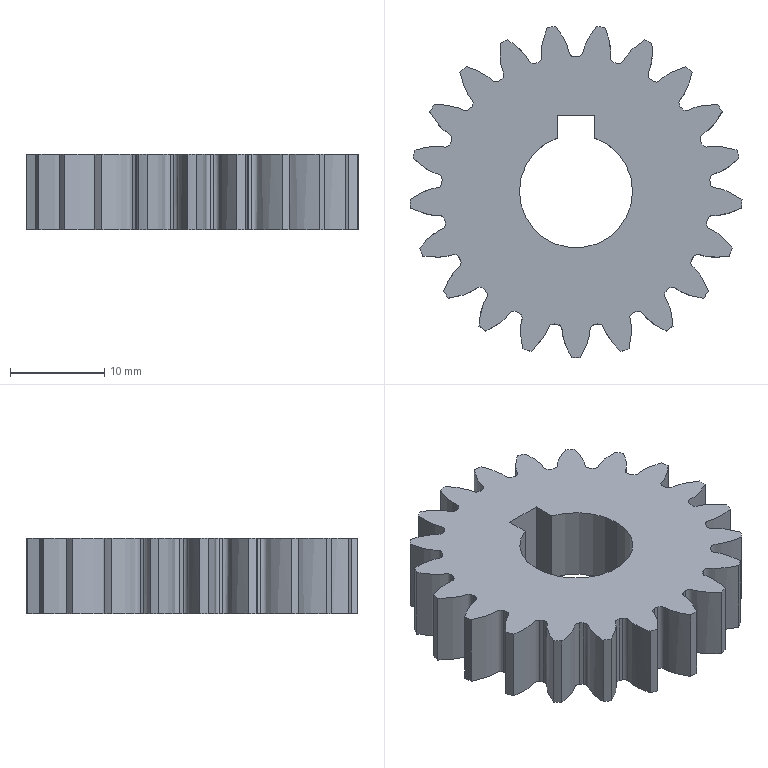Part | SolidWorks | features CirPattern 1, Cut 1, Extrusion 1, ICE 1, RefAxis 1 | 1 solid | 92 faces | box 35.207 x 35.115 x 8 mm | volume 5449 mm3 | cylinder 45 | spline 42 | plane 5 | commonest cylinder face diameters 28.5 x21 35.25 x21 12 x3